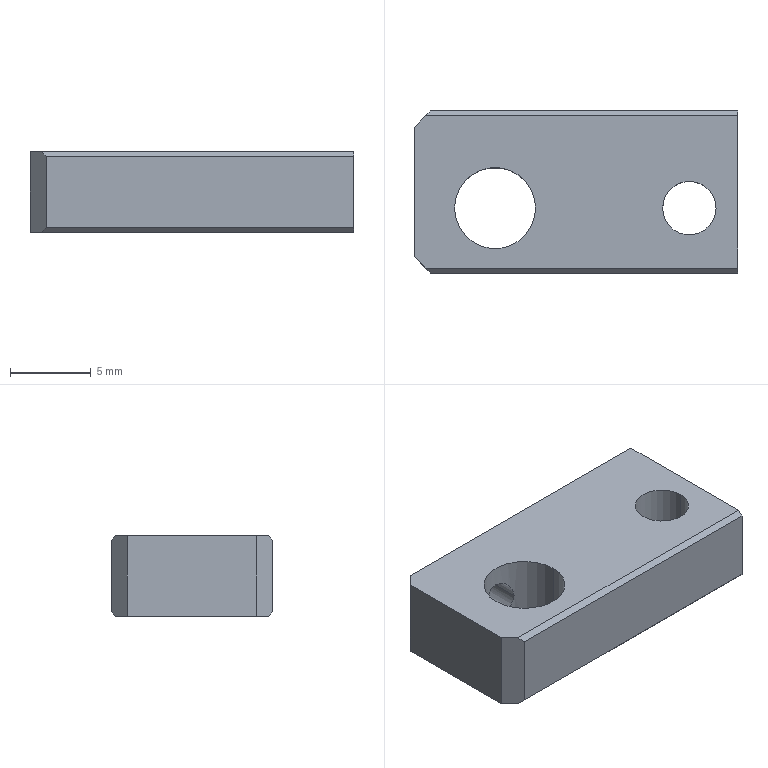Part | NX | 1 solid | 22 faces | box 20 x 10 x 5 mm | volume 831.027 mm3 | plane 12 | cylinder 6 | cone 4 | commonest cylinder face diameters 2.5 x2 3.3 x2 5 x2
STEP:
#1=CARTESIAN_POINT('',(-5.,-3.,5.));
#2=VERTEX_POINT('',#1);
#3=CARTESIAN_POINT('',(-5.,5.,5.));
#4=VERTEX_POINT('',#3);
#5=CARTESIAN_POINT('',(-5.,0.,5.));
#6=DIRECTION('',(0.,1.,0.));
#7=VECTOR('',#6,1000.);
#8=LINE('',#5,#7);
#9=EDGE_CURVE('',#2,#4,#8,.T.);
#10=ORIENTED_EDGE('',*,*,#9,.F.);
#11=CARTESIAN_POINT('',(-4.3,-3.7,5.));
#12=VERTEX_POINT('',#11);
#13=CARTESIAN_POINT('',(-8.,0.,5.));
#14=DIRECTION('',(-0.7071,0.7071,0.));
#15=VECTOR('',#14,1000.);
#16=LINE('',#13,#15);
#17=EDGE_CURVE('',#12,#2,#16,.T.);
#18=ORIENTED_EDGE('',*,*,#17,.F.);
#19=CARTESIAN_POINT('',(15.,-3.7,5.));
#20=VERTEX_POINT('',#19);
#21=CARTESIAN_POINT('',(0.,-3.7,5.));
#22=DIRECTION('',(-1.,0.,0.));
#23=VECTOR('',#22,1000.);
#24=LINE('',#21,#23);
#25=EDGE_CURVE('',#20,#12,#24,.T.);
#26=ORIENTED_EDGE('',*,*,#25,.F.);
#27=CARTESIAN_POINT('',(15.,5.7,5.));
#28=VERTEX_POINT('',#27);
#29=CARTESIAN_POINT('',(15.,0.,5.));
#30=DIRECTION('',(0.,-1.,0.));
#31=VECTOR('',#30,1000.);
#32=LINE('',#29,#31);
#33=EDGE_CURVE('',#28,#20,#32,.T.);
#34=ORIENTED_EDGE('',*,*,#33,.F.);
#35=CARTESIAN_POINT('',(-4.3,5.7,5.));
#36=VERTEX_POINT('',#35);
#37=CARTESIAN_POINT('',(0.,5.7,5.));
#38=DIRECTION('',(-1.,0.,0.));
#39=VECTOR('',#38,1000.);
#40=LINE('',#37,#39);
#41=EDGE_CURVE('',#28,#36,#40,.T.);
#42=ORIENTED_EDGE('',*,*,#41,.T.);
#43=CARTESIAN_POINT('',(-10.,0.,5.));
#44=DIRECTION('',(0.7071,0.7071,0.));
#45=VECTOR('',#44,1000.);
#46=LINE('',#43,#45);
#47=EDGE_CURVE('',#4,#36,#46,.T.);
#48=ORIENTED_EDGE('',*,*,#47,.F.);
#49=EDGE_LOOP('',(#10,#18,#26,#34,#42,#48));
#50=FACE_BOUND('',#49,.T.);
#51=CARTESIAN_POINT('',(-2.5,0.,5.));
#52=VERTEX_POINT('',#51);
#53=CARTESIAN_POINT('',(2.5,0.,5.));
#54=VERTEX_POINT('',#53);
#55=CARTESIAN_POINT('',(0.,0.,5.));
#56=DIRECTION('',(0.,0.,1.));
#57=DIRECTION('',(1.,0.,0.));
#58=AXIS2_PLACEMENT_3D('',#55,#56,#57);
#59=CIRCLE('',#58,2.5);
#60=EDGE_CURVE('',#52,#54,#59,.T.);
#61=ORIENTED_EDGE('',*,*,#60,.F.);
#62=CARTESIAN_POINT('',(0.,0.,5.));
#63=DIRECTION('',(0.,0.,1.));
#64=DIRECTION('',(1.,0.,0.));
#65=AXIS2_PLACEMENT_3D('',#62,#63,#64);
#66=CIRCLE('',#65,2.5);
#67=EDGE_CURVE('',#54,#52,#66,.T.);
#68=ORIENTED_EDGE('',*,*,#67,.F.);
#69=EDGE_LOOP('',(#61,#68));
#70=FACE_BOUND('',#69,.T.);
#71=CARTESIAN_POINT('',(10.35,0.,5.));
#72=VERTEX_POINT('',#71);
#73=CARTESIAN_POINT('',(13.65,0.,5.));
#74=VERTEX_POINT('',#73);
#75=CARTESIAN_POINT('',(12.,0.,5.));
#76=DIRECTION('',(0.,0.,-1.));
#77=DIRECTION('',(-1.,0.,0.));
#78=AXIS2_PLACEMENT_3D('',#75,#76,#77);
#79=CIRCLE('',#78,1.65);
#80=EDGE_CURVE('',#72,#74,#79,.T.);
#81=ORIENTED_EDGE('',*,*,#80,.T.);
#82=CARTESIAN_POINT('',(12.,0.,5.));
#83=DIRECTION('',(0.,0.,-1.));
#84=DIRECTION('',(-1.,0.,0.));
#85=AXIS2_PLACEMENT_3D('',#82,#83,#84);
#86=CIRCLE('',#85,1.65);
#87=EDGE_CURVE('',#74,#72,#86,.T.);
#88=ORIENTED_EDGE('',*,*,#87,.T.);
#89=EDGE_LOOP('',(#81,#88));
#90=FACE_BOUND('',#89,.T.);
#91=CARTESIAN_POINT('',(0.,0.,5.));
#92=DIRECTION('',(0.,0.,1.));
#93=DIRECTION('',(1.,0.,0.));
#94=AXIS2_PLACEMENT_3D('',#91,#92,#93);
#95=PLANE('',#94);
#96=ADVANCED_FACE('',(#50,#70,#90),#95,.T.);
#97=CARTESIAN_POINT('',(-5.,-3.,0.));
#98=VERTEX_POINT('',#97);
#99=CARTESIAN_POINT('',(-5.,5.,0.));
#100=VERTEX_POINT('',#99);
#101=CARTESIAN_POINT('',(-5.,0.,0.));
#102=DIRECTION('',(0.,1.,0.));
#103=VECTOR('',#102,1000.);
#104=LINE('',#101,#103);
#105=EDGE_CURVE('',#98,#100,#104,.T.);
#106=ORIENTED_EDGE('',*,*,#105,.F.);
#107=CARTESIAN_POINT('',(-5.,-3.,5.));
#108=DIRECTION('',(0.,0.,-1.));
#109=VECTOR('',#108,1000.);
#110=LINE('',#107,#109);
#111=EDGE_CURVE('',#2,#98,#110,.T.);
#112=ORIENTED_EDGE('',*,*,#111,.F.);
#113=ORIENTED_EDGE('',*,*,#9,.T.);
#114=CARTESIAN_POINT('',(-5.,5.,5.));
#115=DIRECTION('',(0.,0.,-1.));
#116=VECTOR('',#115,1000.);
#117=LINE('',#114,#116);
#118=EDGE_CURVE('',#4,#100,#117,.T.);
#119=ORIENTED_EDGE('',*,*,#118,.T.);
#120=EDGE_LOOP('',(#106,#112,#113,#119));
#121=FACE_BOUND('',#120,.T.);
#122=CARTESIAN_POINT('',(-5.,6.,0.));
#123=DIRECTION('',(-1.,0.,0.));
#124=DIRECTION('',(0.,0.,1.));
#125=AXIS2_PLACEMENT_3D('',#122,#123,#124);
#126=PLANE('',#125);
#127=ADVANCED_FACE('',(#121),#126,.T.);
#128=ORIENTED_EDGE('',*,*,#118,.F.);
#129=ORIENTED_EDGE('',*,*,#47,.T.);
#130=CARTESIAN_POINT('',(-4.,6.,4.7));
#131=VERTEX_POINT('',#130);
#132=CARTESIAN_POINT('',(0.7,10.7,0.));
#133=DIRECTION('',(0.5774,0.5774,-0.5774));
#134=VECTOR('',#133,1000.);
#135=LINE('',#132,#134);
#136=EDGE_CURVE('',#36,#131,#135,.T.);
#137=ORIENTED_EDGE('',*,*,#136,.T.);
#138=CARTESIAN_POINT('',(-4.,6.,0.3));
#139=VERTEX_POINT('',#138);
#140=CARTESIAN_POINT('',(-4.,6.,0.));
#141=DIRECTION('',(0.,0.,-1.));
#142=VECTOR('',#141,1000.);
#143=LINE('',#140,#142);
#144=EDGE_CURVE('',#131,#139,#143,.T.);
#145=ORIENTED_EDGE('',*,*,#144,.T.);
#146=CARTESIAN_POINT('',(-4.3,5.7,0.));
#147=VERTEX_POINT('',#146);
#148=CARTESIAN_POINT('',(-4.3,5.7,0.));
#149=DIRECTION('',(0.5774,0.5774,0.5774));
#150=VECTOR('',#149,1000.);
#151=LINE('',#148,#150);
#152=EDGE_CURVE('',#147,#139,#151,.T.);
#153=ORIENTED_EDGE('',*,*,#152,.F.);
#154=CARTESIAN_POINT('',(-10.,0.,0.));
#155=DIRECTION('',(0.7071,0.7071,0.));
#156=VECTOR('',#155,1000.);
#157=LINE('',#154,#156);
#158=EDGE_CURVE('',#100,#147,#157,.T.);
#159=ORIENTED_EDGE('',*,*,#158,.F.);
#160=EDGE_LOOP('',(#128,#129,#137,#145,#153,#159));
#161=FACE_BOUND('',#160,.T.);
#162=CARTESIAN_POINT('',(-5.,5.,0.));
#163=DIRECTION('',(-0.7071,0.7071,0.));
#164=DIRECTION('',(0.,0.,1.));
#165=AXIS2_PLACEMENT_3D('',#162,#163,#164);
#166=PLANE('',#165);
#167=ADVANCED_FACE('',(#161),#166,.T.);
#168=CARTESIAN_POINT('',(15.,-3.7,0.));
#169=VERTEX_POINT('',#168);
#170=CARTESIAN_POINT('',(-4.3,-3.7,0.));
#171=VERTEX_POINT('',#170);
#172=CARTESIAN_POINT('',(0.,-3.7,0.));
#173=DIRECTION('',(-1.,0.,0.));
#174=VECTOR('',#173,1000.);
#175=LINE('',#172,#174);
#176=EDGE_CURVE('',#169,#171,#175,.T.);
#177=ORIENTED_EDGE('',*,*,#176,.T.);
#178=CARTESIAN_POINT('',(-8.,0.,0.));
#179=DIRECTION('',(-0.7071,0.7071,0.));
#180=VECTOR('',#179,1000.);
#181=LINE('',#178,#180);
#182=EDGE_CURVE('',#171,#98,#181,.T.);
#183=ORIENTED_EDGE('',*,*,#182,.T.);
#184=ORIENTED_EDGE('',*,*,#105,.T.);
#185=ORIENTED_EDGE('',*,*,#158,.T.);
#186=CARTESIAN_POINT('',(15.,5.7,0.));
#187=VERTEX_POINT('',#186);
#188=CARTESIAN_POINT('',(0.,5.7,0.));
#189=DIRECTION('',(1.,0.,0.));
#190=VECTOR('',#189,1000.);
#191=LINE('',#188,#190);
#192=EDGE_CURVE('',#147,#187,#191,.T.);
#193=ORIENTED_EDGE('',*,*,#192,.T.);
#194=CARTESIAN_POINT('',(15.,0.,0.));
#195=DIRECTION('',(0.,-1.,0.));
#196=VECTOR('',#195,1000.);
#197=LINE('',#194,#196);
#198=EDGE_CURVE('',#187,#169,#197,.T.);
#199=ORIENTED_EDGE('',*,*,#198,.T.);
#200=EDGE_LOOP('',(#177,#183,#184,#185,#193,#199));
#201=FACE_BOUND('',#200,.T.);
#202=CARTESIAN_POINT('',(-2.5,0.,0.));
#203=VERTEX_POINT('',#202);
#204=CARTESIAN_POINT('',(2.5,0.,0.));
#205=VERTEX_POINT('',#204);
#206=CARTESIAN_POINT('',(0.,0.,0.));
#207=DIRECTION('',(0.,0.,1.));
#208=DIRECTION('',(1.,0.,0.));
#209=AXIS2_PLACEMENT_3D('',#206,#207,#208);
#210=CIRCLE('',#209,2.5);
#211=EDGE_CURVE('',#203,#205,#210,.T.);
#212=ORIENTED_EDGE('',*,*,#211,.T.);
#213=CARTESIAN_POINT('',(0.,0.,0.));
#214=DIRECTION('',(0.,0.,1.));
#215=DIRECTION('',(1.,0.,0.));
#216=AXIS2_PLACEMENT_3D('',#213,#214,#215);
#217=CIRCLE('',#216,2.5);
#218=EDGE_CURVE('',#205,#203,#217,.T.);
#219=ORIENTED_EDGE('',*,*,#218,.T.);
#220=EDGE_LOOP('',(#212,#219));
#221=FACE_BOUND('',#220,.T.);
#222=CARTESIAN_POINT('',(14.315,0.,0.));
#223=VERTEX_POINT('',#222);
#224=CARTESIAN_POINT('',(9.685,0.,0.));
#225=VERTEX_POINT('',#224);
#226=CARTESIAN_POINT('',(12.,0.,0.));
#227=DIRECTION('',(0.,0.,-1.));
#228=DIRECTION('',(-1.,0.,0.));
#229=AXIS2_PLACEMENT_3D('',#226,#227,#228);
#230=CIRCLE('',#229,2.315);
#231=EDGE_CURVE('',#223,#225,#230,.T.);
#232=ORIENTED_EDGE('',*,*,#231,.F.);
#233=CARTESIAN_POINT('',(12.,0.,0.));
#234=DIRECTION('',(0.,0.,-1.));
#235=DIRECTION('',(-1.,0.,0.));
#236=AXIS2_PLACEMENT_3D('',#233,#234,#235);
#237=CIRCLE('',#236,2.315);
#238=EDGE_CURVE('',#225,#223,#237,.T.);
#239=ORIENTED_EDGE('',*,*,#238,.F.);
#240=EDGE_LOOP('',(#232,#239));
#241=FACE_BOUND('',#240,.T.);
#242=CARTESIAN_POINT('',(0.,0.,0.));
#243=DIRECTION('',(0.,0.,1.));
#244=DIRECTION('',(1.,0.,0.));
#245=AXIS2_PLACEMENT_3D('',#242,#243,#244);
#246=PLANE('',#245);
#247=ADVANCED_FACE('',(#201,#221,#241),#246,.F.);
#248=ORIENTED_EDGE('',*,*,#198,.F.);
#249=CARTESIAN_POINT('',(15.,6.,0.3));
#250=VERTEX_POINT('',#249);
#251=CARTESIAN_POINT('',(15.,5.7,0.));
#252=DIRECTION('',(0.,-0.7071,-0.7071));
#253=VECTOR('',#252,1000.);
#254=LINE('',#251,#253);
#255=EDGE_CURVE('',#250,#187,#254,.T.);
#256=ORIENTED_EDGE('',*,*,#255,.F.);
#257=CARTESIAN_POINT('',(15.,6.,4.7));
#258=VERTEX_POINT('',#257);
#259=CARTESIAN_POINT('',(15.,6.,0.));
#260=DIRECTION('',(0.,0.,1.));
#261=VECTOR('',#260,1000.);
#262=LINE('',#259,#261);
#263=EDGE_CURVE('',#250,#258,#262,.T.);
#264=ORIENTED_EDGE('',*,*,#263,.T.);
#265=CARTESIAN_POINT('',(15.,10.7,0.));
#266=DIRECTION('',(0.,-0.7071,0.7071));
#267=VECTOR('',#266,1000.);
#268=LINE('',#265,#267);
#269=EDGE_CURVE('',#258,#28,#268,.T.);
#270=ORIENTED_EDGE('',*,*,#269,.T.);
#271=ORIENTED_EDGE('',*,*,#33,.T.);
#272=CARTESIAN_POINT('',(15.,-4.,4.7));
#273=VERTEX_POINT('',#272);
#274=CARTESIAN_POINT('',(15.,-8.7,0.));
#275=DIRECTION('',(0.,0.7071,0.7071));
#276=VECTOR('',#275,1000.);
#277=LINE('',#274,#276);
#278=EDGE_CURVE('',#273,#20,#277,.T.);
#279=ORIENTED_EDGE('',*,*,#278,.F.);
#280=CARTESIAN_POINT('',(15.,-4.,0.3));
#281=VERTEX_POINT('',#280);
#282=CARTESIAN_POINT('',(15.,-4.,5.));
#283=DIRECTION('',(0.,0.,-1.));
#284=VECTOR('',#283,1000.);
#285=LINE('',#282,#284);
#286=EDGE_CURVE('',#273,#281,#285,.T.);
#287=ORIENTED_EDGE('',*,*,#286,.T.);
#288=CARTESIAN_POINT('',(15.,-3.7,0.));
#289=DIRECTION('',(0.,-0.7071,0.7071));
#290=VECTOR('',#289,1000.);
#291=LINE('',#288,#290);
#292=EDGE_CURVE('',#169,#281,#291,.T.);
#293=ORIENTED_EDGE('',*,*,#292,.F.);
#294=EDGE_LOOP('',(#248,#256,#264,#270,#271,#279,#287,#293));
#295=FACE_BOUND('',#294,.T.);
#296=CARTESIAN_POINT('',(15.,-4.,0.));
#297=DIRECTION('',(1.,0.,0.));
#298=DIRECTION('',(0.,1.,0.));
#299=AXIS2_PLACEMENT_3D('',#296,#297,#298);
#300=PLANE('',#299);
#301=ADVANCED_FACE('',(#295),#300,.T.);
#302=CARTESIAN_POINT('',(-4.,-4.,4.7));
#303=VERTEX_POINT('',#302);
#304=CARTESIAN_POINT('',(0.,-4.,4.7));
#305=DIRECTION('',(1.,0.,0.));
#306=VECTOR('',#305,1000.);
#307=LINE('',#304,#306);
#308=EDGE_CURVE('',#303,#273,#307,.T.);
#309=ORIENTED_EDGE('',*,*,#308,.F.);
#310=CARTESIAN_POINT('',(-4.,-4.,0.3));
#311=VERTEX_POINT('',#310);
#312=CARTESIAN_POINT('',(-4.,-4.,5.));
#313=DIRECTION('',(0.,0.,-1.));
#314=VECTOR('',#313,1000.);
#315=LINE('',#312,#314);
#316=EDGE_CURVE('',#303,#311,#315,.T.);
#317=ORIENTED_EDGE('',*,*,#316,.T.);
#318=CARTESIAN_POINT('',(0.,-4.,0.3));
#319=DIRECTION('',(-1.,0.,0.));
#320=VECTOR('',#319,1000.);
#321=LINE('',#318,#320);
#322=EDGE_CURVE('',#281,#311,#321,.T.);
#323=ORIENTED_EDGE('',*,*,#322,.F.);
#324=ORIENTED_EDGE('',*,*,#286,.F.);
#325=EDGE_LOOP('',(#309,#317,#323,#324));
#326=FACE_BOUND('',#325,.T.);
#327=CARTESIAN_POINT('',(-5.,-4.,0.));
#328=DIRECTION('',(0.,-1.,0.));
#329=DIRECTION('',(0.,0.,-1.));
#330=AXIS2_PLACEMENT_3D('',#327,#328,#329);
#331=PLANE('',#330);
#332=ADVANCED_FACE('',(#326),#331,.T.);
#333=ORIENTED_EDGE('',*,*,#316,.F.);
#334=CARTESIAN_POINT('',(0.7,-8.7,0.));
#335=DIRECTION('',(0.5774,-0.5774,-0.5774));
#336=VECTOR('',#335,1000.);
#337=LINE('',#334,#336);
#338=EDGE_CURVE('',#12,#303,#337,.T.);
#339=ORIENTED_EDGE('',*,*,#338,.F.);
#340=ORIENTED_EDGE('',*,*,#17,.T.);
#341=ORIENTED_EDGE('',*,*,#111,.T.);
#342=ORIENTED_EDGE('',*,*,#182,.F.);
#343=CARTESIAN_POINT('',(-4.3,-3.7,0.));
#344=DIRECTION('',(-0.5774,0.5774,-0.5774));
#345=VECTOR('',#344,1000.);
#346=LINE('',#343,#345);
#347=EDGE_CURVE('',#311,#171,#346,.T.);
#348=ORIENTED_EDGE('',*,*,#347,.F.);
#349=EDGE_LOOP('',(#333,#339,#340,#341,#342,#348));
#350=FACE_BOUND('',#349,.T.);
#351=CARTESIAN_POINT('',(-4.,-4.,0.));
#352=DIRECTION('',(-0.7071,-0.7071,0.));
#353=DIRECTION('',(-0.7071,0.7071,0.));
#354=AXIS2_PLACEMENT_3D('',#351,#352,#353);
#355=PLANE('',#354);
#356=ADVANCED_FACE('',(#350),#355,.T.);
#357=CARTESIAN_POINT('',(0.,6.,4.7));
#358=DIRECTION('',(1.,0.,0.));
#359=VECTOR('',#358,1000.);
#360=LINE('',#357,#359);
#361=EDGE_CURVE('',#131,#258,#360,.T.);
#362=ORIENTED_EDGE('',*,*,#361,.T.);
#363=ORIENTED_EDGE('',*,*,#263,.F.);
#364=CARTESIAN_POINT('',(0.,6.,0.3));
#365=DIRECTION('',(1.,0.,0.));
#366=VECTOR('',#365,1000.);
#367=LINE('',#364,#366);
#368=EDGE_CURVE('',#139,#250,#367,.T.);
#369=ORIENTED_EDGE('',*,*,#368,.F.);
#370=ORIENTED_EDGE('',*,*,#144,.F.);
#371=EDGE_LOOP('',(#362,#363,#369,#370));
#372=FACE_BOUND('',#371,.T.);
#373=CARTESIAN_POINT('',(1.7,6.,2.5));
#374=VERTEX_POINT('',#373);
#375=CARTESIAN_POINT('',(-1.7,6.,2.5));
#376=VERTEX_POINT('',#375);
#377=CARTESIAN_POINT('',(0.,6.,2.5));
#378=DIRECTION('',(0.,1.,0.));
#379=DIRECTION('',(1.,0.,0.));
#380=AXIS2_PLACEMENT_3D('',#377,#378,#379);
#381=CIRCLE('',#380,1.7);
#382=EDGE_CURVE('',#374,#376,#381,.T.);
#383=ORIENTED_EDGE('',*,*,#382,.F.);
#384=CARTESIAN_POINT('',(0.,6.,2.5));
#385=DIRECTION('',(0.,1.,0.));
#386=DIRECTION('',(1.,0.,0.));
#387=AXIS2_PLACEMENT_3D('',#384,#385,#386);
#388=CIRCLE('',#387,1.7);
#389=EDGE_CURVE('',#376,#374,#388,.T.);
#390=ORIENTED_EDGE('',*,*,#389,.F.);
#391=EDGE_LOOP('',(#383,#390));
#392=FACE_BOUND('',#391,.T.);
#393=CARTESIAN_POINT('',(15.,6.,0.));
#394=DIRECTION('',(0.,1.,0.));
#395=DIRECTION('',(1.,0.,0.));
#396=AXIS2_PLACEMENT_3D('',#393,#394,#395);
#397=PLANE('',#396);
#398=ADVANCED_FACE('',(#372,#392),#397,.T.);
#399=ORIENTED_EDGE('',*,*,#60,.T.);
#400=CARTESIAN_POINT('',(2.5,0.,0.));
#401=DIRECTION('',(0.,0.,1.));
#402=VECTOR('',#401,1000.);
#403=LINE('',#400,#402);
#404=EDGE_CURVE('',#205,#54,#403,.T.);
#405=ORIENTED_EDGE('',*,*,#404,.F.);
#406=ORIENTED_EDGE('',*,*,#211,.F.);
#407=CARTESIAN_POINT('',(-2.5,0.,0.));
#408=DIRECTION('',(0.,0.,1.));
#409=VECTOR('',#408,1000.);
#410=LINE('',#407,#409);
#411=EDGE_CURVE('',#203,#52,#410,.T.);
#412=ORIENTED_EDGE('',*,*,#411,.T.);
#413=EDGE_LOOP('',(#399,#405,#406,#412));
#414=FACE_BOUND('',#413,.T.);
#415=CARTESIAN_POINT('',(0.,0.,0.));
#416=DIRECTION('',(0.,0.,1.));
#417=DIRECTION('',(1.,0.,0.));
#418=AXIS2_PLACEMENT_3D('',#415,#416,#417);
#419=CYLINDRICAL_SURFACE('',#418,2.5);
#420=ADVANCED_FACE('',(#414),#419,.F.);
#421=ORIENTED_EDGE('',*,*,#361,.F.);
#422=ORIENTED_EDGE('',*,*,#136,.F.);
#423=ORIENTED_EDGE('',*,*,#41,.F.);
#424=ORIENTED_EDGE('',*,*,#269,.F.);
#425=EDGE_LOOP('',(#421,#422,#423,#424));
#426=FACE_BOUND('',#425,.T.);
#427=CARTESIAN_POINT('',(5.5,5.85,4.85));
#428=DIRECTION('',(0.,-0.7071,-0.7071));
#429=DIRECTION('',(0.,-0.7071,0.7071));
#430=AXIS2_PLACEMENT_3D('',#427,#428,#429);
#431=PLANE('',#430);
#432=ADVANCED_FACE('',(#426),#431,.F.);
#433=CARTESIAN_POINT('',(-1.25,2.165,2.5));
#434=VERTEX_POINT('',#433);
#435=CARTESIAN_POINT('',(1.25,2.165,2.5));
#436=VERTEX_POINT('',#435);
#437=CARTESIAN_POINT('',(1.25,2.165,2.5));
#438=CARTESIAN_POINT('',(1.25,2.165,2.654));
#439=CARTESIAN_POINT('',(1.174,2.207,2.959));
#440=CARTESIAN_POINT('',(1.086,2.254,3.132));
#441=CARTESIAN_POINT('',(0.8903,2.34,3.4));
#442=CARTESIAN_POINT('',(0.6605,2.413,3.568));
#443=CARTESIAN_POINT('',(0.4382,2.467,3.684));
#444=CARTESIAN_POINT('',(-0.000141,2.522,3.794));
#445=CARTESIAN_POINT('',(-0.4378,2.467,3.684));
#446=CARTESIAN_POINT('',(-0.6602,2.413,3.568));
#447=CARTESIAN_POINT('',(-0.8904,2.34,3.399));
#448=CARTESIAN_POINT('',(-1.086,2.254,3.132));
#449=CARTESIAN_POINT('',(-1.174,2.207,2.959));
#450=CARTESIAN_POINT('',(-1.25,2.165,2.654));
#451=CARTESIAN_POINT('',(-1.25,2.165,2.5));
#452=B_SPLINE_CURVE_WITH_KNOTS('',3,(#437,#438,#439,#440,#441,#442,#443,#444,#445,#446,#447,#448,#449,#450,#451),.UNSPECIFIED.,.F.,.F.,(4,1,1,1,1,1,1,1,1,1,1,1,4),(0.,0.125,0.1875,0.25,0.3125,0.375,0.5,0.625,0.6875,0.75,0.8125,0.875,1.),.UNSPECIFIED.);
#453=EDGE_CURVE('',#434,#436,#452,.F.);
#454=ORIENTED_EDGE('',*,*,#453,.F.);
#455=CARTESIAN_POINT('',(-1.25,5.74,2.5));
#456=VERTEX_POINT('',#455);
#457=CARTESIAN_POINT('',(-1.25,6.,2.5));
#458=DIRECTION('',(0.,1.,0.));
#459=VECTOR('',#458,1000.);
#460=LINE('',#457,#459);
#461=EDGE_CURVE('',#456,#434,#460,.F.);
#462=ORIENTED_EDGE('',*,*,#461,.F.);
#463=CARTESIAN_POINT('',(1.25,5.74,2.5));
#464=VERTEX_POINT('',#463);
#465=CARTESIAN_POINT('',(0.,5.74,2.5));
#466=DIRECTION('',(0.,1.,0.));
#467=DIRECTION('',(1.,0.,0.));
#468=AXIS2_PLACEMENT_3D('',#465,#466,#467);
#469=CIRCLE('',#468,1.25);
#470=EDGE_CURVE('',#456,#464,#469,.T.);
#471=ORIENTED_EDGE('',*,*,#470,.T.);
#472=CARTESIAN_POINT('',(1.25,6.,2.5));
#473=DIRECTION('',(0.,1.,0.));
#474=VECTOR('',#473,1000.);
#475=LINE('',#472,#474);
#476=EDGE_CURVE('',#464,#436,#475,.F.);
#477=ORIENTED_EDGE('',*,*,#476,.T.);
#478=EDGE_LOOP('',(#454,#462,#471,#477));
#479=FACE_BOUND('',#478,.T.);
#480=CARTESIAN_POINT('',(0.,6.,2.5));
#481=DIRECTION('',(0.,1.,0.));
#482=DIRECTION('',(1.,0.,0.));
#483=AXIS2_PLACEMENT_3D('',#480,#481,#482);
#484=CYLINDRICAL_SURFACE('',#483,1.25);
#485=ADVANCED_FACE('',(#479),#484,.F.);
#486=CARTESIAN_POINT('',(0.,5.74,2.5));
#487=DIRECTION('',(0.,1.,0.));
#488=DIRECTION('',(1.,0.,0.));
#489=AXIS2_PLACEMENT_3D('',#486,#487,#488);
#490=CIRCLE('',#489,1.25);
#491=EDGE_CURVE('',#464,#456,#490,.T.);
#492=ORIENTED_EDGE('',*,*,#491,.F.);
#493=CARTESIAN_POINT('',(1.25,5.74,2.5));
#494=DIRECTION('',(0.866,0.5,0.));
#495=VECTOR('',#494,1000.);
#496=LINE('',#493,#495);
#497=EDGE_CURVE('',#464,#374,#496,.T.);
#498=ORIENTED_EDGE('',*,*,#497,.T.);
#499=ORIENTED_EDGE('',*,*,#382,.T.);
#500=CARTESIAN_POINT('',(-1.25,5.74,2.5));
#501=DIRECTION('',(-0.866,0.5,0.));
#502=VECTOR('',#501,1000.);
#503=LINE('',#500,#502);
#504=EDGE_CURVE('',#456,#376,#503,.T.);
#505=ORIENTED_EDGE('',*,*,#504,.F.);
#506=EDGE_LOOP('',(#492,#498,#499,#505));
#507=FACE_BOUND('',#506,.T.);
#508=CARTESIAN_POINT('',(0.,5.74,2.5));
#509=DIRECTION('',(0.,1.,0.));
#510=DIRECTION('',(1.,0.,0.));
#511=AXIS2_PLACEMENT_3D('',#508,#509,#510);
#512=CONICAL_SURFACE('',#511,1.25,1.047);
#513=ADVANCED_FACE('',(#507),#512,.F.);
#514=ORIENTED_EDGE('',*,*,#368,.T.);
#515=ORIENTED_EDGE('',*,*,#255,.T.);
#516=ORIENTED_EDGE('',*,*,#192,.F.);
#517=ORIENTED_EDGE('',*,*,#152,.T.);
#518=EDGE_LOOP('',(#514,#515,#516,#517));
#519=FACE_BOUND('',#518,.T.);
#520=CARTESIAN_POINT('',(5.5,5.85,0.15));
#521=DIRECTION('',(0.,0.7071,-0.7071));
#522=DIRECTION('',(-1.,0.,0.));
#523=AXIS2_PLACEMENT_3D('',#520,#521,#522);
#524=PLANE('',#523);
#525=ADVANCED_FACE('',(#519),#524,.T.);
#526=ORIENTED_EDGE('',*,*,#176,.F.);
#527=ORIENTED_EDGE('',*,*,#292,.T.);
#528=ORIENTED_EDGE('',*,*,#322,.T.);
#529=ORIENTED_EDGE('',*,*,#347,.T.);
#530=EDGE_LOOP('',(#526,#527,#528,#529));
#531=FACE_BOUND('',#530,.T.);
#532=CARTESIAN_POINT('',(5.5,-3.85,0.15));
#533=DIRECTION('',(0.,-0.7071,-0.7071));
#534=DIRECTION('',(0.,0.7071,-0.7071));
#535=AXIS2_PLACEMENT_3D('',#532,#533,#534);
#536=PLANE('',#535);
#537=ADVANCED_FACE('',(#531),#536,.T.);
#538=ORIENTED_EDGE('',*,*,#308,.T.);
#539=ORIENTED_EDGE('',*,*,#278,.T.);
#540=ORIENTED_EDGE('',*,*,#25,.T.);
#541=ORIENTED_EDGE('',*,*,#338,.T.);
#542=EDGE_LOOP('',(#538,#539,#540,#541));
#543=FACE_BOUND('',#542,.T.);
#544=CARTESIAN_POINT('',(5.5,-3.85,4.85));
#545=DIRECTION('',(0.,-0.7071,0.7071));
#546=DIRECTION('',(-1.,0.,0.));
#547=AXIS2_PLACEMENT_3D('',#544,#545,#546);
#548=PLANE('',#547);
#549=ADVANCED_FACE('',(#543),#548,.T.);
#550=CARTESIAN_POINT('',(10.35,0.,0.3839));
#551=VERTEX_POINT('',#550);
#552=CARTESIAN_POINT('',(13.65,0.,0.3839));
#553=VERTEX_POINT('',#552);
#554=CARTESIAN_POINT('',(12.,0.,0.3839));
#555=DIRECTION('',(0.,0.,-1.));
#556=DIRECTION('',(-1.,0.,0.));
#557=AXIS2_PLACEMENT_3D('',#554,#555,#556);
#558=CIRCLE('',#557,1.65);
#559=EDGE_CURVE('',#551,#553,#558,.T.);
#560=ORIENTED_EDGE('',*,*,#559,.T.);
#561=CARTESIAN_POINT('',(13.65,0.,0.));
#562=DIRECTION('',(0.,0.,-1.));
#563=VECTOR('',#562,1000.);
#564=LINE('',#561,#563);
#565=EDGE_CURVE('',#553,#74,#564,.F.);
#566=ORIENTED_EDGE('',*,*,#565,.T.);
#567=ORIENTED_EDGE('',*,*,#80,.F.);
#568=CARTESIAN_POINT('',(10.35,0.,0.));
#569=DIRECTION('',(0.,0.,-1.));
#570=VECTOR('',#569,1000.);
#571=LINE('',#568,#570);
#572=EDGE_CURVE('',#551,#72,#571,.F.);
#573=ORIENTED_EDGE('',*,*,#572,.F.);
#574=EDGE_LOOP('',(#560,#566,#567,#573));
#575=FACE_BOUND('',#574,.T.);
#576=CARTESIAN_POINT('',(12.,0.,0.));
#577=DIRECTION('',(0.,0.,-1.));
#578=DIRECTION('',(-1.,0.,0.));
#579=AXIS2_PLACEMENT_3D('',#576,#577,#578);
#580=CYLINDRICAL_SURFACE('',#579,1.65);
#581=ADVANCED_FACE('',(#575),#580,.F.);
#582=ORIENTED_EDGE('',*,*,#231,.T.);
#583=CARTESIAN_POINT('',(10.35,0.,0.3839));
#584=DIRECTION('',(-0.866,0.,-0.5));
#585=VECTOR('',#584,1000.);
#586=LINE('',#583,#585);
#587=EDGE_CURVE('',#225,#551,#586,.F.);
#588=ORIENTED_EDGE('',*,*,#587,.T.);
#589=CARTESIAN_POINT('',(12.,0.,0.3839));
#590=DIRECTION('',(0.,0.,-1.));
#591=DIRECTION('',(-1.,0.,0.));
#592=AXIS2_PLACEMENT_3D('',#589,#590,#591);
#593=CIRCLE('',#592,1.65);
#594=EDGE_CURVE('',#553,#551,#593,.T.);
#595=ORIENTED_EDGE('',*,*,#594,.F.);
#596=CARTESIAN_POINT('',(13.65,0.,0.3839));
#597=DIRECTION('',(0.866,0.,-0.5));
#598=VECTOR('',#597,1000.);
#599=LINE('',#596,#598);
#600=EDGE_CURVE('',#223,#553,#599,.F.);
#601=ORIENTED_EDGE('',*,*,#600,.F.);
#602=EDGE_LOOP('',(#582,#588,#595,#601));
#603=FACE_BOUND('',#602,.T.);
#604=CARTESIAN_POINT('',(12.,0.,0.3839));
#605=DIRECTION('',(0.,0.,-1.));
#606=DIRECTION('',(-1.,0.,0.));
#607=AXIS2_PLACEMENT_3D('',#604,#605,#606);
#608=CONICAL_SURFACE('',#607,1.65,1.047);
#609=ADVANCED_FACE('',(#603),#608,.F.);
#610=ORIENTED_EDGE('',*,*,#497,.F.);
#611=ORIENTED_EDGE('',*,*,#470,.F.);
#612=ORIENTED_EDGE('',*,*,#504,.T.);
#613=ORIENTED_EDGE('',*,*,#389,.T.);
#614=EDGE_LOOP('',(#610,#611,#612,#613));
#615=FACE_BOUND('',#614,.T.);
#616=CARTESIAN_POINT('',(0.,5.74,2.5));
#617=DIRECTION('',(0.,1.,0.));
#618=DIRECTION('',(1.,0.,0.));
#619=AXIS2_PLACEMENT_3D('',#616,#617,#618);
#620=CONICAL_SURFACE('',#619,1.25,1.047);
#621=ADVANCED_FACE('',(#615),#620,.F.);
#622=ORIENTED_EDGE('',*,*,#572,.T.);
#623=ORIENTED_EDGE('',*,*,#87,.F.);
#624=ORIENTED_EDGE('',*,*,#565,.F.);
#625=ORIENTED_EDGE('',*,*,#594,.T.);
#626=EDGE_LOOP('',(#622,#623,#624,#625));
#627=FACE_BOUND('',#626,.T.);
#628=CARTESIAN_POINT('',(12.,0.,0.));
#629=DIRECTION('',(0.,0.,-1.));
#630=DIRECTION('',(-1.,0.,0.));
#631=AXIS2_PLACEMENT_3D('',#628,#629,#630);
#632=CYLINDRICAL_SURFACE('',#631,1.65);
#633=ADVANCED_FACE('',(#627),#632,.F.);
#634=ORIENTED_EDGE('',*,*,#404,.T.);
#635=ORIENTED_EDGE('',*,*,#67,.T.);
#636=ORIENTED_EDGE('',*,*,#411,.F.);
#637=ORIENTED_EDGE('',*,*,#218,.F.);
#638=EDGE_LOOP('',(#634,#635,#636,#637));
#639=FACE_BOUND('',#638,.T.);
#640=ORIENTED_EDGE('',*,*,#453,.T.);
#641=CARTESIAN_POINT('',(1.25,2.165,2.5));
#642=CARTESIAN_POINT('',(1.25,2.165,2.169));
#643=CARTESIAN_POINT('',(0.9812,2.344,1.524));
#644=CARTESIAN_POINT('',(-0.00008612,2.578,1.113));
#645=CARTESIAN_POINT('',(-0.9809,2.344,1.524));
#646=CARTESIAN_POINT('',(-1.25,2.165,2.169));
#647=CARTESIAN_POINT('',(-1.25,2.165,2.5));
#648=B_SPLINE_CURVE_WITH_KNOTS('',3,(#641,#642,#643,#644,#645,#646,#647),.UNSPECIFIED.,.F.,.F.,(4,1,1,1,4),(0.,0.25,0.5,0.75,1.),.UNSPECIFIED.);
#649=EDGE_CURVE('',#436,#434,#648,.T.);
#650=ORIENTED_EDGE('',*,*,#649,.T.);
#651=EDGE_LOOP('',(#640,#650));
#652=FACE_BOUND('',#651,.T.);
#653=CARTESIAN_POINT('',(0.,0.,0.));
#654=DIRECTION('',(0.,0.,1.));
#655=DIRECTION('',(1.,0.,0.));
#656=AXIS2_PLACEMENT_3D('',#653,#654,#655);
#657=CYLINDRICAL_SURFACE('',#656,2.5);
#658=ADVANCED_FACE('',(#639,#652),#657,.F.);
#659=ORIENTED_EDGE('',*,*,#559,.F.);
#660=ORIENTED_EDGE('',*,*,#587,.F.);
#661=ORIENTED_EDGE('',*,*,#238,.T.);
#662=ORIENTED_EDGE('',*,*,#600,.T.);
#663=EDGE_LOOP('',(#659,#660,#661,#662));
#664=FACE_BOUND('',#663,.T.);
#665=CARTESIAN_POINT('',(12.,0.,0.3839));
#666=DIRECTION('',(0.,0.,-1.));
#667=DIRECTION('',(-1.,0.,0.));
#668=AXIS2_PLACEMENT_3D('',#665,#666,#667);
#669=CONICAL_SURFACE('',#668,1.65,1.047);
#670=ADVANCED_FACE('',(#664),#669,.F.);
#671=ORIENTED_EDGE('',*,*,#491,.T.);
#672=ORIENTED_EDGE('',*,*,#461,.T.);
#673=ORIENTED_EDGE('',*,*,#649,.F.);
#674=ORIENTED_EDGE('',*,*,#476,.F.);
#675=EDGE_LOOP('',(#671,#672,#673,#674));
#676=FACE_BOUND('',#675,.T.);
#677=CARTESIAN_POINT('',(0.,6.,2.5));
#678=DIRECTION('',(0.,1.,0.));
#679=DIRECTION('',(1.,0.,0.));
#680=AXIS2_PLACEMENT_3D('',#677,#678,#679);
#681=CYLINDRICAL_SURFACE('',#680,1.25);
#682=ADVANCED_FACE('',(#676),#681,.F.);
#683=CLOSED_SHELL('',(#96,#127,#167,#247,#301,#332,#356,#398,#420,#432,#485,#513,#525,#537,#549,#581,#609,#621,#633,#658,#670,#682));
#684=MANIFOLD_SOLID_BREP('',#683);
#685=(LENGTH_UNIT()NAMED_UNIT(*)SI_UNIT(.MILLI.,.METRE.));
#686=UNCERTAINTY_MEASURE_WITH_UNIT(LENGTH_MEASURE(0.0508),#685,'','');
#687=(NAMED_UNIT(*)PLANE_ANGLE_UNIT()SI_UNIT($,.RADIAN.));
#688=(NAMED_UNIT(*)SI_UNIT($,.STERADIAN.)SOLID_ANGLE_UNIT());
#689=(GEOMETRIC_REPRESENTATION_CONTEXT(3)GLOBAL_UNCERTAINTY_ASSIGNED_CONTEXT((#686))GLOBAL_UNIT_ASSIGNED_CONTEXT((#685,#687,#688))REPRESENTATION_CONTEXT('',''));
#690=ADVANCED_BREP_SHAPE_REPRESENTATION('',(#684),#689);